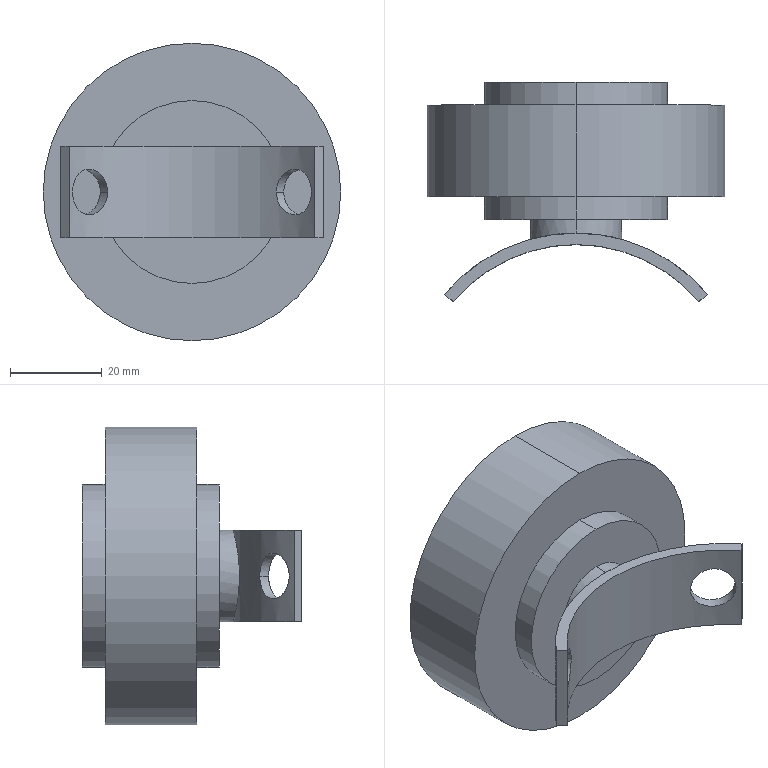Part | SolidWorks | features ICE 5, RevCut 2, Extrusion 1 | 1 solid | 26 faces | box 65 x 48.002 x 65 mm | volume 76467 mm3 | cylinder 17 | plane 9 | commonest cylinder face diameters 10 x4 20 x4 40 x4 65 x2 75 x2 70 x1
STEP:
#1=CARTESIAN_POINT('',(27.72,25.256,10.));
#2=VERTEX_POINT('',#1);
#3=CARTESIAN_POINT('',(20.059,31.684,10.));
#4=VERTEX_POINT('',#3);
#5=CARTESIAN_POINT('',(27.72,25.256,10.));
#6=CARTESIAN_POINT('',(27.72,25.256,9.669));
#7=CARTESIAN_POINT('',(27.697,25.281,9.344));
#8=CARTESIAN_POINT('',(27.632,25.351,8.864));
#9=CARTESIAN_POINT('',(27.605,25.381,8.706));
#10=CARTESIAN_POINT('',(27.54,25.452,8.392));
#11=CARTESIAN_POINT('',(27.502,25.493,8.235));
#12=CARTESIAN_POINT('',(27.373,25.632,7.781));
#13=CARTESIAN_POINT('',(27.267,25.745,7.494));
#14=CARTESIAN_POINT('',(27.015,26.009,6.951));
#15=CARTESIAN_POINT('',(26.868,26.162,6.694));
#16=CARTESIAN_POINT('',(26.543,26.491,6.233));
#17=CARTESIAN_POINT('',(26.364,26.67,6.027));
#18=CARTESIAN_POINT('',(25.971,27.052,5.661));
#19=CARTESIAN_POINT('',(25.761,27.253,5.506));
#20=CARTESIAN_POINT('',(25.32,27.663,5.257));
#21=CARTESIAN_POINT('',(25.086,27.876,5.16));
#22=CARTESIAN_POINT('',(24.602,28.304,5.032));
#23=CARTESIAN_POINT('',(24.356,28.516,5.));
#24=CARTESIAN_POINT('',(23.856,28.935,5.));
#25=CARTESIAN_POINT('',(23.599,29.145,5.032));
#26=CARTESIAN_POINT('',(23.097,29.545,5.16));
#27=CARTESIAN_POINT('',(22.85,29.736,5.255));
#28=CARTESIAN_POINT('',(22.487,30.01,5.443));
#29=CARTESIAN_POINT('',(22.367,30.1,5.514));
#30=CARTESIAN_POINT('',(22.133,30.272,5.669));
#31=CARTESIAN_POINT('',(22.02,30.354,5.753));
#32=CARTESIAN_POINT('',(21.689,30.592,6.024));
#33=CARTESIAN_POINT('',(21.482,30.738,6.231));
#34=CARTESIAN_POINT('',(21.096,31.004,6.697));
#35=CARTESIAN_POINT('',(20.924,31.12,6.95));
#36=CARTESIAN_POINT('',(20.697,31.272,7.355));
#37=CARTESIAN_POINT('',(20.626,31.318,7.495));
#38=CARTESIAN_POINT('',(20.495,31.404,7.785));
#39=CARTESIAN_POINT('',(20.436,31.443,7.935));
#40=CARTESIAN_POINT('',(20.276,31.546,8.389));
#41=CARTESIAN_POINT('',(20.196,31.597,8.7));
#42=CARTESIAN_POINT('',(20.087,31.666,9.342));
#43=CARTESIAN_POINT('',(20.059,31.684,9.673));
#44=CARTESIAN_POINT('',(20.059,31.684,10.));
#45=B_SPLINE_CURVE_WITH_KNOTS('',3,(#5,#6,#7,#8,#9,#10,#11,#12,#13,#14,#15,#16,#17,#18,#19,#20,#21,#22,#23,#24,#25,#26,#27,#28,#29,#30,#31,#32,#33,#34,#35,#36,#37,#38,#39,#40,#41,#42,#43,#44),.UNSPECIFIED.,.F.,.F.,(4,2,2,2,2,2,2,2,2,2,2,2,2,2,2,2,2,2,2,4),(0.,0.0009781,0.001467,0.001956,0.002934,0.003912,0.004891,0.005869,0.006847,0.007825,0.008803,0.009781,0.01027,0.01076,0.01174,0.01272,0.0132,0.01369,0.01467,0.01565),.UNSPECIFIED.);
#46=EDGE_CURVE('',#2,#4,#45,.T.);
#47=ORIENTED_EDGE('',*,*,#46,.T.);
#48=CARTESIAN_POINT('',(18.437,29.75,10.));
#49=VERTEX_POINT('',#48);
#50=CARTESIAN_POINT('',(13.962,24.418,10.));
#51=DIRECTION('',(-0.6428,-0.766,0.));
#52=VECTOR('',#51,1000.);
#53=LINE('',#50,#52);
#54=EDGE_CURVE('',#4,#49,#53,.T.);
#55=ORIENTED_EDGE('',*,*,#54,.T.);
#56=CARTESIAN_POINT('',(26.097,23.323,10.));
#57=VERTEX_POINT('',#56);
#58=CARTESIAN_POINT('',(18.437,29.75,10.));
#59=CARTESIAN_POINT('',(18.437,29.75,9.674));
#60=CARTESIAN_POINT('',(18.464,29.734,9.349));
#61=CARTESIAN_POINT('',(18.574,29.665,8.703));
#62=CARTESIAN_POINT('',(18.656,29.614,8.388));
#63=CARTESIAN_POINT('',(18.868,29.479,7.786));
#64=CARTESIAN_POINT('',(19.,29.394,7.495));
#65=CARTESIAN_POINT('',(19.308,29.193,6.949));
#66=CARTESIAN_POINT('',(19.481,29.078,6.697));
#67=CARTESIAN_POINT('',(19.864,28.818,6.236));
#68=CARTESIAN_POINT('',(20.076,28.671,6.025));
#69=CARTESIAN_POINT('',(20.519,28.356,5.662));
#70=CARTESIAN_POINT('',(20.751,28.186,5.509));
#71=CARTESIAN_POINT('',(21.115,27.914,5.32));
#72=CARTESIAN_POINT('',(21.24,27.819,5.264));
#73=CARTESIAN_POINT('',(21.489,27.627,5.168));
#74=CARTESIAN_POINT('',(21.613,27.53,5.129));
#75=CARTESIAN_POINT('',(21.989,27.232,5.033));
#76=CARTESIAN_POINT('',(22.242,27.026,5.));
#77=CARTESIAN_POINT('',(22.748,26.601,5.));
#78=CARTESIAN_POINT('',(22.994,26.389,5.032));
#79=CARTESIAN_POINT('',(23.473,25.964,5.159));
#80=CARTESIAN_POINT('',(23.708,25.749,5.255));
#81=CARTESIAN_POINT('',(24.15,25.335,5.506));
#82=CARTESIAN_POINT('',(24.358,25.135,5.659));
#83=CARTESIAN_POINT('',(24.746,24.753,6.021));
#84=CARTESIAN_POINT('',(24.928,24.57,6.232));
#85=CARTESIAN_POINT('',(25.251,24.238,6.692));
#86=CARTESIAN_POINT('',(25.394,24.087,6.943));
#87=CARTESIAN_POINT('',(25.647,23.818,7.49));
#88=CARTESIAN_POINT('',(25.753,23.703,7.78));
#89=CARTESIAN_POINT('',(25.923,23.517,8.381));
#90=CARTESIAN_POINT('',(25.988,23.444,8.696));
#91=CARTESIAN_POINT('',(26.075,23.347,9.342));
#92=CARTESIAN_POINT('',(26.097,23.323,9.669));
#93=CARTESIAN_POINT('',(26.097,23.323,10.));
#94=B_SPLINE_CURVE_WITH_KNOTS('',3,(#58,#59,#60,#61,#62,#63,#64,#65,#66,#67,#68,#69,#70,#71,#72,#73,#74,#75,#76,#77,#78,#79,#80,#81,#82,#83,#84,#85,#86,#87,#88,#89,#90,#91,#92,#93),.UNSPECIFIED.,.F.,.F.,(4,2,2,2,2,2,2,2,2,2,2,2,2,2,2,2,2,4),(0.01565,0.01663,0.01761,0.01859,0.01956,0.02054,0.02152,0.02201,0.0225,0.02348,0.02445,0.02543,0.02641,0.02739,0.02837,0.02934,0.03032,0.0313),.UNSPECIFIED.);
#95=EDGE_CURVE('',#49,#57,#94,.T.);
#96=ORIENTED_EDGE('',*,*,#95,.T.);
#97=CARTESIAN_POINT('',(21.623,17.991,10.));
#98=DIRECTION('',(-0.6428,-0.766,0.));
#99=VECTOR('',#98,1000.);
#100=LINE('',#97,#99);
#101=EDGE_CURVE('',#2,#57,#100,.T.);
#102=ORIENTED_EDGE('',*,*,#101,.F.);
#103=EDGE_LOOP('',(#47,#55,#96,#102));
#104=FACE_OUTER_BOUND('',#103,.T.);
#105=CARTESIAN_POINT('',(17.793,21.204,10.));
#106=DIRECTION('',(-0.6428,-0.766,0.));
#107=DIRECTION('',(0.766,-0.6428,0.));
#108=AXIS2_PLACEMENT_3D('',#105,#106,#107);
#109=CYLINDRICAL_SURFACE('',#108,5.);
#110=ADVANCED_FACE('',(#104),#109,.F.);
#111=CARTESIAN_POINT('',(-20.059,31.684,10.));
#112=VERTEX_POINT('',#111);
#113=CARTESIAN_POINT('',(-27.72,25.256,10.));
#114=VERTEX_POINT('',#113);
#115=CARTESIAN_POINT('',(-20.059,31.684,10.));
#116=CARTESIAN_POINT('',(-20.059,31.684,9.669));
#117=CARTESIAN_POINT('',(-20.087,31.667,9.344));
#118=CARTESIAN_POINT('',(-20.168,31.615,8.864));
#119=CARTESIAN_POINT('',(-20.202,31.593,8.706));
#120=CARTESIAN_POINT('',(-20.283,31.541,8.392));
#121=CARTESIAN_POINT('',(-20.33,31.511,8.235));
#122=CARTESIAN_POINT('',(-20.489,31.408,7.781));
#123=CARTESIAN_POINT('',(-20.619,31.323,7.494));
#124=CARTESIAN_POINT('',(-20.923,31.121,6.951));
#125=CARTESIAN_POINT('',(-21.099,31.002,6.694));
#126=CARTESIAN_POINT('',(-21.48,30.74,6.233));
#127=CARTESIAN_POINT('',(-21.687,30.594,6.027));
#128=CARTESIAN_POINT('',(-22.131,30.274,5.661));
#129=CARTESIAN_POINT('',(-22.366,30.102,5.506));
#130=CARTESIAN_POINT('',(-22.846,29.739,5.257));
#131=CARTESIAN_POINT('',(-23.096,29.545,5.16));
#132=CARTESIAN_POINT('',(-23.601,29.143,5.032));
#133=CARTESIAN_POINT('',(-23.853,28.938,5.));
#134=CARTESIAN_POINT('',(-24.353,28.518,5.));
#135=CARTESIAN_POINT('',(-24.605,28.301,5.032));
#136=CARTESIAN_POINT('',(-25.085,27.876,5.16));
#137=CARTESIAN_POINT('',(-25.316,27.666,5.255));
#138=CARTESIAN_POINT('',(-25.649,27.357,5.443));
#139=CARTESIAN_POINT('',(-25.759,27.254,5.514));
#140=CARTESIAN_POINT('',(-25.969,27.054,5.669));
#141=CARTESIAN_POINT('',(-26.07,26.956,5.753));
#142=CARTESIAN_POINT('',(-26.361,26.672,6.024));
#143=CARTESIAN_POINT('',(-26.541,26.493,6.231));
#144=CARTESIAN_POINT('',(-26.87,26.16,6.697));
#145=CARTESIAN_POINT('',(-27.014,26.01,6.95));
#146=CARTESIAN_POINT('',(-27.203,25.812,7.355));
#147=CARTESIAN_POINT('',(-27.261,25.751,7.495));
#148=CARTESIAN_POINT('',(-27.368,25.637,7.785));
#149=CARTESIAN_POINT('',(-27.416,25.585,7.935));
#150=CARTESIAN_POINT('',(-27.545,25.446,8.389));
#151=CARTESIAN_POINT('',(-27.61,25.376,8.7));
#152=CARTESIAN_POINT('',(-27.697,25.281,9.342));
#153=CARTESIAN_POINT('',(-27.72,25.256,9.673));
#154=CARTESIAN_POINT('',(-27.72,25.256,10.));
#155=B_SPLINE_CURVE_WITH_KNOTS('',3,(#115,#116,#117,#118,#119,#120,#121,#122,#123,#124,#125,#126,#127,#128,#129,#130,#131,#132,#133,#134,#135,#136,#137,#138,#139,#140,#141,#142,#143,#144,#145,#146,#147,#148,#149,#150,#151,#152,#153,#154),.UNSPECIFIED.,.F.,.F.,(4,2,2,2,2,2,2,2,2,2,2,2,2,2,2,2,2,2,2,4),(0.,0.0009781,0.001467,0.001956,0.002934,0.003912,0.004891,0.005869,0.006847,0.007825,0.008803,0.009781,0.01027,0.01076,0.01174,0.01272,0.0132,0.01369,0.01467,0.01565),.UNSPECIFIED.);
#156=EDGE_CURVE('',#112,#114,#155,.T.);
#157=ORIENTED_EDGE('',*,*,#156,.T.);
#158=CARTESIAN_POINT('',(-26.097,23.323,10.));
#159=VERTEX_POINT('',#158);
#160=CARTESIAN_POINT('',(-21.523,17.872,10.));
#161=DIRECTION('',(0.6428,-0.766,0.));
#162=VECTOR('',#161,1000.);
#163=LINE('',#160,#162);
#164=EDGE_CURVE('',#114,#159,#163,.T.);
#165=ORIENTED_EDGE('',*,*,#164,.T.);
#166=CARTESIAN_POINT('',(-18.437,29.75,10.));
#167=VERTEX_POINT('',#166);
#168=CARTESIAN_POINT('',(-26.097,23.323,10.));
#169=CARTESIAN_POINT('',(-26.097,23.323,9.674));
#170=CARTESIAN_POINT('',(-26.076,23.347,9.349));
#171=CARTESIAN_POINT('',(-25.989,23.443,8.703));
#172=CARTESIAN_POINT('',(-25.924,23.515,8.388));
#173=CARTESIAN_POINT('',(-25.755,23.7,7.786));
#174=CARTESIAN_POINT('',(-25.649,23.816,7.495));
#175=CARTESIAN_POINT('',(-25.397,24.084,6.949));
#176=CARTESIAN_POINT('',(-25.254,24.234,6.697));
#177=CARTESIAN_POINT('',(-24.931,24.566,6.236));
#178=CARTESIAN_POINT('',(-24.75,24.749,6.025));
#179=CARTESIAN_POINT('',(-24.362,25.131,5.662));
#180=CARTESIAN_POINT('',(-24.155,25.331,5.509));
#181=CARTESIAN_POINT('',(-23.823,25.642,5.32));
#182=CARTESIAN_POINT('',(-23.708,25.748,5.264));
#183=CARTESIAN_POINT('',(-23.476,25.959,5.168));
#184=CARTESIAN_POINT('',(-23.358,26.066,5.129));
#185=CARTESIAN_POINT('',(-23.,26.384,5.033));
#186=CARTESIAN_POINT('',(-22.753,26.597,5.));
#187=CARTESIAN_POINT('',(-22.247,27.022,5.));
#188=CARTESIAN_POINT('',(-21.995,27.227,5.032));
#189=CARTESIAN_POINT('',(-21.493,27.625,5.159));
#190=CARTESIAN_POINT('',(-21.241,27.819,5.255));
#191=CARTESIAN_POINT('',(-20.756,28.183,5.506));
#192=CARTESIAN_POINT('',(-20.524,28.352,5.659));
#193=CARTESIAN_POINT('',(-20.08,28.669,6.021));
#194=CARTESIAN_POINT('',(-19.868,28.815,6.232));
#195=CARTESIAN_POINT('',(-19.485,29.076,6.692));
#196=CARTESIAN_POINT('',(-19.311,29.191,6.943));
#197=CARTESIAN_POINT('',(-19.002,29.393,7.49));
#198=CARTESIAN_POINT('',(-18.871,29.477,7.78));
#199=CARTESIAN_POINT('',(-18.658,29.612,8.381));
#200=CARTESIAN_POINT('',(-18.575,29.664,8.696));
#201=CARTESIAN_POINT('',(-18.465,29.733,9.342));
#202=CARTESIAN_POINT('',(-18.437,29.75,9.669));
#203=CARTESIAN_POINT('',(-18.437,29.75,10.));
#204=B_SPLINE_CURVE_WITH_KNOTS('',3,(#168,#169,#170,#171,#172,#173,#174,#175,#176,#177,#178,#179,#180,#181,#182,#183,#184,#185,#186,#187,#188,#189,#190,#191,#192,#193,#194,#195,#196,#197,#198,#199,#200,#201,#202,#203),.UNSPECIFIED.,.F.,.F.,(4,2,2,2,2,2,2,2,2,2,2,2,2,2,2,2,2,4),(0.01565,0.01663,0.01761,0.01859,0.01956,0.02054,0.02152,0.02201,0.0225,0.02348,0.02445,0.02543,0.02641,0.02739,0.02837,0.02934,0.03032,0.0313),.UNSPECIFIED.);
#205=EDGE_CURVE('',#159,#167,#204,.T.);
#206=ORIENTED_EDGE('',*,*,#205,.T.);
#207=CARTESIAN_POINT('',(-13.863,24.3,10.));
#208=DIRECTION('',(0.6428,-0.766,0.));
#209=VECTOR('',#208,1000.);
#210=LINE('',#207,#209);
#211=EDGE_CURVE('',#112,#167,#210,.T.);
#212=ORIENTED_EDGE('',*,*,#211,.F.);
#213=EDGE_LOOP('',(#157,#165,#206,#212));
#214=FACE_OUTER_BOUND('',#213,.T.);
#215=CARTESIAN_POINT('',(-17.693,21.086,10.));
#216=DIRECTION('',(0.6428,-0.766,0.));
#217=DIRECTION('',(0.766,0.6428,0.));
#218=AXIS2_PLACEMENT_3D('',#215,#216,#217);
#219=CYLINDRICAL_SURFACE('',#218,5.);
#220=ADVANCED_FACE('',(#214),#219,.F.);
#221=CARTESIAN_POINT('',(0.,50.5,0.));
#222=VERTEX_POINT('',#221);
#223=CARTESIAN_POINT('',(0.,50.5,20.));
#224=VERTEX_POINT('',#223);
#225=CARTESIAN_POINT('',(0.,50.5,10.));
#226=DIRECTION('',(0.,1.,0.));
#227=DIRECTION('',(0.,0.,1.));
#228=AXIS2_PLACEMENT_3D('',#225,#226,#227);
#229=CIRCLE('',#228,10.);
#230=EDGE_CURVE('',#222,#224,#229,.T.);
#231=ORIENTED_EDGE('',*,*,#230,.F.);
#232=CARTESIAN_POINT('',(0.,70.5,0.));
#233=VERTEX_POINT('',#232);
#234=CARTESIAN_POINT('',(0.,50.5,0.));
#235=DIRECTION('',(0.,1.,0.));
#236=VECTOR('',#235,1000.);
#237=LINE('',#234,#236);
#238=EDGE_CURVE('',#222,#233,#237,.T.);
#239=ORIENTED_EDGE('',*,*,#238,.T.);
#240=CARTESIAN_POINT('',(0.,70.5,20.));
#241=VERTEX_POINT('',#240);
#242=CARTESIAN_POINT('',(0.,70.5,10.));
#243=DIRECTION('',(0.,1.,0.));
#244=DIRECTION('',(0.,0.,1.));
#245=AXIS2_PLACEMENT_3D('',#242,#243,#244);
#246=CIRCLE('',#245,10.);
#247=EDGE_CURVE('',#233,#241,#246,.T.);
#248=ORIENTED_EDGE('',*,*,#247,.T.);
#249=CARTESIAN_POINT('',(0.,50.5,20.));
#250=DIRECTION('',(0.,1.,0.));
#251=VECTOR('',#250,1000.);
#252=LINE('',#249,#251);
#253=EDGE_CURVE('',#224,#241,#252,.T.);
#254=ORIENTED_EDGE('',*,*,#253,.F.);
#255=EDGE_LOOP('',(#231,#239,#248,#254));
#256=FACE_OUTER_BOUND('',#255,.T.);
#257=CARTESIAN_POINT('',(0.,50.5,10.));
#258=DIRECTION('',(0.,1.,0.));
#259=DIRECTION('',(0.,0.,1.));
#260=AXIS2_PLACEMENT_3D('',#257,#258,#259);
#261=CYLINDRICAL_SURFACE('',#260,10.);
#262=ADVANCED_FACE('',(#256),#261,.F.);
#263=CARTESIAN_POINT('',(0.,70.5,30.));
#264=VERTEX_POINT('',#263);
#265=CARTESIAN_POINT('',(0.,70.5,-10.));
#266=VERTEX_POINT('',#265);
#267=CARTESIAN_POINT('',(0.,70.5,10.));
#268=DIRECTION('',(0.,1.,0.));
#269=DIRECTION('',(0.,0.,1.));
#270=AXIS2_PLACEMENT_3D('',#267,#268,#269);
#271=CIRCLE('',#270,20.);
#272=EDGE_CURVE('',#264,#266,#271,.T.);
#273=ORIENTED_EDGE('',*,*,#272,.F.);
#274=CARTESIAN_POINT('',(0.,65.5,30.));
#275=VERTEX_POINT('',#274);
#276=CARTESIAN_POINT('',(0.,70.5,30.));
#277=DIRECTION('',(0.,-1.,0.));
#278=VECTOR('',#277,1000.);
#279=LINE('',#276,#278);
#280=EDGE_CURVE('',#264,#275,#279,.T.);
#281=ORIENTED_EDGE('',*,*,#280,.T.);
#282=CARTESIAN_POINT('',(0.,65.5,-10.));
#283=VERTEX_POINT('',#282);
#284=CARTESIAN_POINT('',(0.,65.5,10.));
#285=DIRECTION('',(0.,1.,0.));
#286=DIRECTION('',(0.,0.,1.));
#287=AXIS2_PLACEMENT_3D('',#284,#285,#286);
#288=CIRCLE('',#287,20.);
#289=EDGE_CURVE('',#275,#283,#288,.T.);
#290=ORIENTED_EDGE('',*,*,#289,.T.);
#291=CARTESIAN_POINT('',(0.,70.5,-10.));
#292=DIRECTION('',(0.,-1.,0.));
#293=VECTOR('',#292,1000.);
#294=LINE('',#291,#293);
#295=EDGE_CURVE('',#266,#283,#294,.T.);
#296=ORIENTED_EDGE('',*,*,#295,.F.);
#297=EDGE_LOOP('',(#273,#281,#290,#296));
#298=FACE_OUTER_BOUND('',#297,.T.);
#299=CARTESIAN_POINT('',(0.,70.5,10.));
#300=DIRECTION('',(0.,-1.,0.));
#301=DIRECTION('',(0.,0.,-1.));
#302=AXIS2_PLACEMENT_3D('',#299,#300,#301);
#303=CYLINDRICAL_SURFACE('',#302,20.);
#304=ADVANCED_FACE('',(#298),#303,.T.);
#305=CARTESIAN_POINT('',(0.,65.5,42.5));
#306=VERTEX_POINT('',#305);
#307=CARTESIAN_POINT('',(0.,65.5,-22.5));
#308=VERTEX_POINT('',#307);
#309=CARTESIAN_POINT('',(0.,65.5,10.));
#310=DIRECTION('',(0.,1.,0.));
#311=DIRECTION('',(0.,0.,1.));
#312=AXIS2_PLACEMENT_3D('',#309,#310,#311);
#313=CIRCLE('',#312,32.5);
#314=EDGE_CURVE('',#306,#308,#313,.T.);
#315=ORIENTED_EDGE('',*,*,#314,.F.);
#316=CARTESIAN_POINT('',(0.,45.5,42.5));
#317=VERTEX_POINT('',#316);
#318=CARTESIAN_POINT('',(0.,65.5,42.5));
#319=DIRECTION('',(0.,-1.,0.));
#320=VECTOR('',#319,1000.);
#321=LINE('',#318,#320);
#322=EDGE_CURVE('',#306,#317,#321,.T.);
#323=ORIENTED_EDGE('',*,*,#322,.T.);
#324=CARTESIAN_POINT('',(0.,45.5,-22.5));
#325=VERTEX_POINT('',#324);
#326=CARTESIAN_POINT('',(0.,45.5,10.));
#327=DIRECTION('',(0.,1.,0.));
#328=DIRECTION('',(0.,0.,1.));
#329=AXIS2_PLACEMENT_3D('',#326,#327,#328);
#330=CIRCLE('',#329,32.5);
#331=EDGE_CURVE('',#317,#325,#330,.T.);
#332=ORIENTED_EDGE('',*,*,#331,.T.);
#333=CARTESIAN_POINT('',(0.,65.5,-22.5));
#334=DIRECTION('',(0.,-1.,0.));
#335=VECTOR('',#334,1000.);
#336=LINE('',#333,#335);
#337=EDGE_CURVE('',#308,#325,#336,.T.);
#338=ORIENTED_EDGE('',*,*,#337,.F.);
#339=EDGE_LOOP('',(#315,#323,#332,#338));
#340=FACE_OUTER_BOUND('',#339,.T.);
#341=CARTESIAN_POINT('',(0.,65.5,10.));
#342=DIRECTION('',(0.,-1.,0.));
#343=DIRECTION('',(0.,0.,-1.));
#344=AXIS2_PLACEMENT_3D('',#341,#342,#343);
#345=CYLINDRICAL_SURFACE('',#344,32.5);
#346=ADVANCED_FACE('',(#340),#345,.T.);
#347=CARTESIAN_POINT('',(0.,45.5,30.));
#348=VERTEX_POINT('',#347);
#349=CARTESIAN_POINT('',(0.,45.5,-10.));
#350=VERTEX_POINT('',#349);
#351=CARTESIAN_POINT('',(0.,45.5,10.));
#352=DIRECTION('',(0.,1.,0.));
#353=DIRECTION('',(0.,0.,1.));
#354=AXIS2_PLACEMENT_3D('',#351,#352,#353);
#355=CIRCLE('',#354,20.);
#356=EDGE_CURVE('',#348,#350,#355,.T.);
#357=ORIENTED_EDGE('',*,*,#356,.F.);
#358=CARTESIAN_POINT('',(0.,40.5,30.));
#359=VERTEX_POINT('',#358);
#360=CARTESIAN_POINT('',(0.,45.5,30.));
#361=DIRECTION('',(0.,-1.,0.));
#362=VECTOR('',#361,1000.);
#363=LINE('',#360,#362);
#364=EDGE_CURVE('',#348,#359,#363,.T.);
#365=ORIENTED_EDGE('',*,*,#364,.T.);
#366=CARTESIAN_POINT('',(0.,40.5,-10.));
#367=VERTEX_POINT('',#366);
#368=CARTESIAN_POINT('',(0.,40.5,10.));
#369=DIRECTION('',(0.,1.,0.));
#370=DIRECTION('',(0.,0.,1.));
#371=AXIS2_PLACEMENT_3D('',#368,#369,#370);
#372=CIRCLE('',#371,20.);
#373=EDGE_CURVE('',#359,#367,#372,.T.);
#374=ORIENTED_EDGE('',*,*,#373,.T.);
#375=CARTESIAN_POINT('',(0.,45.5,-10.));
#376=DIRECTION('',(0.,-1.,0.));
#377=VECTOR('',#376,1000.);
#378=LINE('',#375,#377);
#379=EDGE_CURVE('',#350,#367,#378,.T.);
#380=ORIENTED_EDGE('',*,*,#379,.F.);
#381=EDGE_LOOP('',(#357,#365,#374,#380));
#382=FACE_OUTER_BOUND('',#381,.T.);
#383=CARTESIAN_POINT('',(0.,45.5,10.));
#384=DIRECTION('',(0.,-1.,0.));
#385=DIRECTION('',(0.,0.,-1.));
#386=AXIS2_PLACEMENT_3D('',#383,#384,#385);
#387=CYLINDRICAL_SURFACE('',#386,20.);
#388=ADVANCED_FACE('',(#382),#387,.T.);
#389=CARTESIAN_POINT('',(0.,37.5,20.));
#390=VERTEX_POINT('',#389);
#391=CARTESIAN_POINT('',(0.,37.5,0.));
#392=VERTEX_POINT('',#391);
#393=CARTESIAN_POINT('',(0.,37.5,20.));
#394=CARTESIAN_POINT('',(0.664,37.5,20.));
#395=CARTESIAN_POINT('',(1.316,37.482,19.935));
#396=CARTESIAN_POINT('',(2.278,37.432,19.743));
#397=CARTESIAN_POINT('',(2.596,37.411,19.663));
#398=CARTESIAN_POINT('',(3.226,37.362,19.471));
#399=CARTESIAN_POINT('',(3.538,37.334,19.359));
#400=CARTESIAN_POINT('',(4.445,37.241,18.982));
#401=CARTESIAN_POINT('',(5.019,37.167,18.674));
#402=CARTESIAN_POINT('',(5.832,37.045,18.13));
#403=CARTESIAN_POINT('',(6.097,37.002,17.933));
#404=CARTESIAN_POINT('',(6.603,36.915,17.517));
#405=CARTESIAN_POINT('',(6.844,36.871,17.298));
#406=CARTESIAN_POINT('',(7.532,36.739,16.61));
#407=CARTESIAN_POINT('',(7.945,36.651,16.108));
#408=CARTESIAN_POINT('',(8.493,36.526,15.289));
#409=CARTESIAN_POINT('',(8.662,36.486,15.007));
#410=CARTESIAN_POINT('',(8.97,36.412,14.432));
#411=CARTESIAN_POINT('',(9.109,36.377,14.138));
#412=CARTESIAN_POINT('',(9.359,36.314,13.537));
#413=CARTESIAN_POINT('',(9.47,36.285,13.23));
#414=CARTESIAN_POINT('',(9.661,36.234,12.603));
#415=CARTESIAN_POINT('',(9.742,36.212,12.28));
#416=CARTESIAN_POINT('',(9.936,36.16,11.311));
#417=CARTESIAN_POINT('',(10.,36.142,10.66));
#418=CARTESIAN_POINT('',(10.,36.142,9.349));
#419=CARTESIAN_POINT('',(9.934,36.16,8.683));
#420=CARTESIAN_POINT('',(9.678,36.23,7.398));
#421=CARTESIAN_POINT('',(9.488,36.281,6.773));
#422=CARTESIAN_POINT('',(9.11,36.377,5.862));
#423=CARTESIAN_POINT('',(8.968,36.412,5.563));
#424=CARTESIAN_POINT('',(8.659,36.487,4.987));
#425=CARTESIAN_POINT('',(8.491,36.527,4.708));
#426=CARTESIAN_POINT('',(8.13,36.609,4.168));
#427=CARTESIAN_POINT('',(7.936,36.651,3.907));
#428=CARTESIAN_POINT('',(7.522,36.738,3.403));
#429=CARTESIAN_POINT('',(7.301,36.783,3.158));
#430=CARTESIAN_POINT('',(6.606,36.916,2.465));
#431=CARTESIAN_POINT('',(6.105,37.004,2.053));
#432=CARTESIAN_POINT('',(5.294,37.125,1.51));
#433=CARTESIAN_POINT('',(5.014,37.164,1.342));
#434=CARTESIAN_POINT('',(4.434,37.238,1.031));
#435=CARTESIAN_POINT('',(4.136,37.272,0.8896));
#436=CARTESIAN_POINT('',(3.231,37.365,0.5139));
#437=CARTESIAN_POINT('',(2.608,37.415,0.3236));
#438=CARTESIAN_POINT('',(1.641,37.465,0.13));
#439=CARTESIAN_POINT('',(1.311,37.479,0.08085));
#440=CARTESIAN_POINT('',(0.6549,37.496,0.01602));
#441=CARTESIAN_POINT('',(0.3272,37.5,0.));
#442=CARTESIAN_POINT('',(0.,37.5,0.));
#443=B_SPLINE_CURVE_WITH_KNOTS('',3,(#393,#394,#395,#396,#397,#398,#399,#400,#401,#402,#403,#404,#405,#406,#407,#408,#409,#410,#411,#412,#413,#414,#415,#416,#417,#418,#419,#420,#421,#422,#423,#424,#425,#426,#427,#428,#429,#430,#431,#432,#433,#434,#435,#436,#437,#438,#439,#440,#441,#442),.UNSPECIFIED.,.F.,.F.,(4,2,2,2,2,2,2,2,2,2,2,2,2,2,2,2,2,2,2,2,2,2,2,2,4),(0.,0.001963,0.002944,0.003926,0.005889,0.00687,0.007852,0.009815,0.0108,0.01178,0.01276,0.01374,0.0157,0.01767,0.01963,0.02061,0.02159,0.02257,0.02356,0.02552,0.0265,0.02748,0.02944,0.03043,0.03141),.UNSPECIFIED.);
#444=EDGE_CURVE('',#390,#392,#443,.T.);
#445=ORIENTED_EDGE('',*,*,#444,.T.);
#446=CARTESIAN_POINT('',(0.,40.5,0.));
#447=VERTEX_POINT('',#446);
#448=CARTESIAN_POINT('',(0.,22.496,0.));
#449=DIRECTION('',(0.,1.,0.));
#450=VECTOR('',#449,1000.);
#451=LINE('',#448,#450);
#452=EDGE_CURVE('',#392,#447,#451,.T.);
#453=ORIENTED_EDGE('',*,*,#452,.T.);
#454=CARTESIAN_POINT('',(0.,40.5,20.));
#455=VERTEX_POINT('',#454);
#456=CARTESIAN_POINT('',(0.,40.5,10.));
#457=DIRECTION('',(0.,1.,0.));
#458=DIRECTION('',(0.,0.,1.));
#459=AXIS2_PLACEMENT_3D('',#456,#457,#458);
#460=CIRCLE('',#459,10.);
#461=EDGE_CURVE('',#455,#447,#460,.T.);
#462=ORIENTED_EDGE('',*,*,#461,.F.);
#463=CARTESIAN_POINT('',(0.,22.496,20.));
#464=DIRECTION('',(0.,1.,0.));
#465=VECTOR('',#464,1000.);
#466=LINE('',#463,#465);
#467=EDGE_CURVE('',#390,#455,#466,.T.);
#468=ORIENTED_EDGE('',*,*,#467,.F.);
#469=EDGE_LOOP('',(#445,#453,#462,#468));
#470=FACE_OUTER_BOUND('',#469,.T.);
#471=CARTESIAN_POINT('',(0.,22.496,10.));
#472=DIRECTION('',(0.,1.,0.));
#473=DIRECTION('',(0.,0.,1.));
#474=AXIS2_PLACEMENT_3D('',#471,#472,#473);
#475=CYLINDRICAL_SURFACE('',#474,10.);
#476=ADVANCED_FACE('',(#470),#475,.T.);
#477=CARTESIAN_POINT('',(-26.812,22.498,0.));
#478=VERTEX_POINT('',#477);
#479=CARTESIAN_POINT('',(26.812,22.498,0.));
#480=VERTEX_POINT('',#479);
#481=CARTESIAN_POINT('',(0.,0.,0.));
#482=DIRECTION('',(0.,0.,-1.));
#483=DIRECTION('',(1.,0.,0.));
#484=AXIS2_PLACEMENT_3D('',#481,#482,#483);
#485=CIRCLE('',#484,35.);
#486=EDGE_CURVE('',#478,#480,#485,.T.);
#487=ORIENTED_EDGE('',*,*,#486,.T.);
#488=CARTESIAN_POINT('',(26.812,22.498,20.));
#489=VERTEX_POINT('',#488);
#490=CARTESIAN_POINT('',(26.812,22.498,20.));
#491=DIRECTION('',(0.,0.,-1.));
#492=VECTOR('',#491,1000.);
#493=LINE('',#490,#492);
#494=EDGE_CURVE('',#489,#480,#493,.T.);
#495=ORIENTED_EDGE('',*,*,#494,.F.);
#496=CARTESIAN_POINT('',(-26.812,22.498,20.));
#497=VERTEX_POINT('',#496);
#498=CARTESIAN_POINT('',(0.,0.,20.));
#499=DIRECTION('',(0.,0.,-1.));
#500=DIRECTION('',(1.,0.,0.));
#501=AXIS2_PLACEMENT_3D('',#498,#499,#500);
#502=CIRCLE('',#501,35.);
#503=EDGE_CURVE('',#497,#489,#502,.T.);
#504=ORIENTED_EDGE('',*,*,#503,.F.);
#505=CARTESIAN_POINT('',(-26.812,22.498,20.));
#506=DIRECTION('',(0.,0.,-1.));
#507=VECTOR('',#506,1000.);
#508=LINE('',#505,#507);
#509=EDGE_CURVE('',#497,#478,#508,.T.);
#510=ORIENTED_EDGE('',*,*,#509,.T.);
#511=EDGE_LOOP('',(#487,#495,#504,#510));
#512=FACE_OUTER_BOUND('',#511,.T.);
#513=CARTESIAN_POINT('',(-18.437,29.75,10.));
#514=CARTESIAN_POINT('',(-18.437,29.75,10.331));
#515=CARTESIAN_POINT('',(-18.465,29.733,10.656));
#516=CARTESIAN_POINT('',(-18.546,29.682,11.136));
#517=CARTESIAN_POINT('',(-18.58,29.661,11.294));
#518=CARTESIAN_POINT('',(-18.662,29.61,11.609));
#519=CARTESIAN_POINT('',(-18.71,29.58,11.765));
#520=CARTESIAN_POINT('',(-18.87,29.478,12.219));
#521=CARTESIAN_POINT('',(-19.,29.394,12.506));
#522=CARTESIAN_POINT('',(-19.306,29.194,13.049));
#523=CARTESIAN_POINT('',(-19.483,29.077,13.306));
#524=CARTESIAN_POINT('',(-19.866,28.816,13.767));
#525=CARTESIAN_POINT('',(-20.074,28.673,13.973));
#526=CARTESIAN_POINT('',(-20.52,28.355,14.339));
#527=CARTESIAN_POINT('',(-20.756,28.183,14.494));
#528=CARTESIAN_POINT('',(-21.238,27.822,14.743));
#529=CARTESIAN_POINT('',(-21.488,27.629,14.84));
#530=CARTESIAN_POINT('',(-21.994,27.228,14.968));
#531=CARTESIAN_POINT('',(-22.246,27.023,15.));
#532=CARTESIAN_POINT('',(-22.746,26.603,15.));
#533=CARTESIAN_POINT('',(-22.997,26.386,14.967));
#534=CARTESIAN_POINT('',(-23.477,25.96,14.84));
#535=CARTESIAN_POINT('',(-23.708,25.749,14.745));
#536=CARTESIAN_POINT('',(-24.04,25.438,14.557));
#537=CARTESIAN_POINT('',(-24.149,25.335,14.486));
#538=CARTESIAN_POINT('',(-24.358,25.134,14.331));
#539=CARTESIAN_POINT('',(-24.458,25.036,14.247));
#540=CARTESIAN_POINT('',(-24.749,24.75,13.976));
#541=CARTESIAN_POINT('',(-24.927,24.57,13.769));
#542=CARTESIAN_POINT('',(-25.254,24.234,13.303));
#543=CARTESIAN_POINT('',(-25.397,24.083,13.051));
#544=CARTESIAN_POINT('',(-25.647,23.818,12.509));
#545=CARTESIAN_POINT('',(-25.754,23.701,12.217));
#546=CARTESIAN_POINT('',(-25.925,23.515,11.612));
#547=CARTESIAN_POINT('',(-25.989,23.444,11.3));
#548=CARTESIAN_POINT('',(-26.075,23.347,10.658));
#549=CARTESIAN_POINT('',(-26.097,23.323,10.327));
#550=CARTESIAN_POINT('',(-26.097,23.323,10.));
#551=B_SPLINE_CURVE_WITH_KNOTS('',3,(#513,#514,#515,#516,#517,#518,#519,#520,#521,#522,#523,#524,#525,#526,#527,#528,#529,#530,#531,#532,#533,#534,#535,#536,#537,#538,#539,#540,#541,#542,#543,#544,#545,#546,#547,#548,#549,#550),.UNSPECIFIED.,.F.,.F.,(4,2,2,2,2,2,2,2,2,2,2,2,2,2,2,2,2,2,4),(0.,0.0009783,0.001467,0.001957,0.002935,0.003913,0.004891,0.00587,0.006848,0.007826,0.008804,0.009783,0.01027,0.01076,0.01174,0.01272,0.0137,0.01467,0.01565),.UNSPECIFIED.);
#552=EDGE_CURVE('',#167,#159,#551,.T.);
#553=ORIENTED_EDGE('',*,*,#552,.F.);
#554=ORIENTED_EDGE('',*,*,#205,.F.);
#555=EDGE_LOOP('',(#553,#554));
#556=FACE_BOUND('',#555,.T.);
#557=CARTESIAN_POINT('',(26.097,23.323,10.));
#558=CARTESIAN_POINT('',(26.097,23.323,10.331));
#559=CARTESIAN_POINT('',(26.075,23.347,10.656));
#560=CARTESIAN_POINT('',(26.011,23.419,11.136));
#561=CARTESIAN_POINT('',(25.984,23.449,11.294));
#562=CARTESIAN_POINT('',(25.919,23.52,11.609));
#563=CARTESIAN_POINT('',(25.881,23.562,11.765));
#564=CARTESIAN_POINT('',(25.753,23.702,12.219));
#565=CARTESIAN_POINT('',(25.648,23.816,12.506));
#566=CARTESIAN_POINT('',(25.398,24.083,13.049));
#567=CARTESIAN_POINT('',(25.252,24.236,13.306));
#568=CARTESIAN_POINT('',(24.929,24.568,13.767));
#569=CARTESIAN_POINT('',(24.751,24.748,13.973));
#570=CARTESIAN_POINT('',(24.361,25.132,14.339));
#571=CARTESIAN_POINT('',(24.151,25.334,14.494));
#572=CARTESIAN_POINT('',(23.711,25.746,14.743));
#573=CARTESIAN_POINT('',(23.478,25.959,14.84));
#574=CARTESIAN_POINT('',(22.995,26.388,14.968));
#575=CARTESIAN_POINT('',(22.749,26.6,15.));
#576=CARTESIAN_POINT('',(22.249,27.02,15.));
#577=CARTESIAN_POINT('',(21.992,27.23,14.967));
#578=CARTESIAN_POINT('',(21.489,27.629,14.84));
#579=CARTESIAN_POINT('',(21.241,27.819,14.745));
#580=CARTESIAN_POINT('',(20.877,28.092,14.557));
#581=CARTESIAN_POINT('',(20.756,28.181,14.486));
#582=CARTESIAN_POINT('',(20.522,28.352,14.331));
#583=CARTESIAN_POINT('',(20.408,28.434,14.247));
#584=CARTESIAN_POINT('',(20.077,28.671,13.976));
#585=CARTESIAN_POINT('',(19.868,28.815,13.769));
#586=CARTESIAN_POINT('',(19.481,29.079,13.303));
#587=CARTESIAN_POINT('',(19.307,29.193,13.051));
#588=CARTESIAN_POINT('',(19.002,29.393,12.509));
#589=CARTESIAN_POINT('',(18.869,29.478,12.217));
#590=CARTESIAN_POINT('',(18.656,29.614,11.612));
#591=CARTESIAN_POINT('',(18.575,29.665,11.3));
#592=CARTESIAN_POINT('',(18.465,29.733,10.658));
#593=CARTESIAN_POINT('',(18.437,29.75,10.327));
#594=CARTESIAN_POINT('',(18.437,29.75,10.));
#595=B_SPLINE_CURVE_WITH_KNOTS('',3,(#557,#558,#559,#560,#561,#562,#563,#564,#565,#566,#567,#568,#569,#570,#571,#572,#573,#574,#575,#576,#577,#578,#579,#580,#581,#582,#583,#584,#585,#586,#587,#588,#589,#590,#591,#592,#593,#594),.UNSPECIFIED.,.F.,.F.,(4,2,2,2,2,2,2,2,2,2,2,2,2,2,2,2,2,2,4),(0.,0.0009783,0.001467,0.001957,0.002935,0.003913,0.004891,0.00587,0.006848,0.007826,0.008804,0.009783,0.01027,0.01076,0.01174,0.01272,0.0137,0.01467,0.01565),.UNSPECIFIED.);
#596=EDGE_CURVE('',#57,#49,#595,.T.);
#597=ORIENTED_EDGE('',*,*,#596,.F.);
#598=ORIENTED_EDGE('',*,*,#95,.F.);
#599=EDGE_LOOP('',(#597,#598));
#600=FACE_BOUND('',#599,.T.);
#601=CARTESIAN_POINT('',(0.,0.,20.));
#602=DIRECTION('',(0.,0.,-1.));
#603=DIRECTION('',(-1.,0.,0.));
#604=AXIS2_PLACEMENT_3D('',#601,#602,#603);
#605=CYLINDRICAL_SURFACE('',#604,35.);
#606=ADVANCED_FACE('',(#512,#556,#600),#605,.F.);
#607=CARTESIAN_POINT('',(28.727,24.105,0.));
#608=VERTEX_POINT('',#607);
#609=CARTESIAN_POINT('',(0.,0.,0.));
#610=DIRECTION('',(0.,0.,1.));
#611=DIRECTION('',(1.,0.,0.));
#612=AXIS2_PLACEMENT_3D('',#609,#610,#611);
#613=CIRCLE('',#612,37.5);
#614=EDGE_CURVE('',#608,#392,#613,.T.);
#615=ORIENTED_EDGE('',*,*,#614,.T.);
#616=ORIENTED_EDGE('',*,*,#444,.F.);
#617=CARTESIAN_POINT('',(28.727,24.105,20.));
#618=VERTEX_POINT('',#617);
#619=CARTESIAN_POINT('',(0.,0.,20.));
#620=DIRECTION('',(0.,0.,1.));
#621=DIRECTION('',(1.,0.,0.));
#622=AXIS2_PLACEMENT_3D('',#619,#620,#621);
#623=CIRCLE('',#622,37.5);
#624=EDGE_CURVE('',#618,#390,#623,.T.);
#625=ORIENTED_EDGE('',*,*,#624,.F.);
#626=CARTESIAN_POINT('',(28.727,24.105,20.));
#627=DIRECTION('',(0.,0.,-1.));
#628=VECTOR('',#627,1000.);
#629=LINE('',#626,#628);
#630=EDGE_CURVE('',#618,#608,#629,.T.);
#631=ORIENTED_EDGE('',*,*,#630,.T.);
#632=EDGE_LOOP('',(#615,#616,#625,#631));
#633=FACE_OUTER_BOUND('',#632,.T.);
#634=ORIENTED_EDGE('',*,*,#46,.F.);
#635=CARTESIAN_POINT('',(20.059,31.684,10.));
#636=CARTESIAN_POINT('',(20.059,31.684,10.326));
#637=CARTESIAN_POINT('',(20.086,31.667,10.651));
#638=CARTESIAN_POINT('',(20.195,31.598,11.297));
#639=CARTESIAN_POINT('',(20.277,31.545,11.612));
#640=CARTESIAN_POINT('',(20.488,31.409,12.214));
#641=CARTESIAN_POINT('',(20.619,31.323,12.505));
#642=CARTESIAN_POINT('',(20.924,31.12,13.051));
#643=CARTESIAN_POINT('',(21.096,31.004,13.303));
#644=CARTESIAN_POINT('',(21.477,30.741,13.764));
#645=CARTESIAN_POINT('',(21.688,30.593,13.975));
#646=CARTESIAN_POINT('',(22.13,30.275,14.338));
#647=CARTESIAN_POINT('',(22.361,30.105,14.491));
#648=CARTESIAN_POINT('',(22.724,29.831,14.68));
#649=CARTESIAN_POINT('',(22.848,29.736,14.736));
#650=CARTESIAN_POINT('',(23.097,29.544,14.832));
#651=CARTESIAN_POINT('',(23.221,29.446,14.871));
#652=CARTESIAN_POINT('',(23.597,29.147,14.967));
#653=CARTESIAN_POINT('',(23.849,28.941,15.));
#654=CARTESIAN_POINT('',(24.355,28.516,15.));
#655=CARTESIAN_POINT('',(24.601,28.304,14.968));
#656=CARTESIAN_POINT('',(25.081,27.88,14.841));
#657=CARTESIAN_POINT('',(25.316,27.666,14.745));
#658=CARTESIAN_POINT('',(25.76,27.254,14.495));
#659=CARTESIAN_POINT('',(25.968,27.055,14.341));
#660=CARTESIAN_POINT('',(26.359,26.675,13.979));
#661=CARTESIAN_POINT('',(26.541,26.493,13.768));
#662=CARTESIAN_POINT('',(26.866,26.163,13.308));
#663=CARTESIAN_POINT('',(27.011,26.013,13.057));
#664=CARTESIAN_POINT('',(27.265,25.747,12.51));
#665=CARTESIAN_POINT('',(27.372,25.633,12.22));
#666=CARTESIAN_POINT('',(27.544,25.448,11.619));
#667=CARTESIAN_POINT('',(27.609,25.377,11.304));
#668=CARTESIAN_POINT('',(27.697,25.28,10.658));
#669=CARTESIAN_POINT('',(27.72,25.256,10.331));
#670=CARTESIAN_POINT('',(27.72,25.256,10.));
#671=B_SPLINE_CURVE_WITH_KNOTS('',3,(#635,#636,#637,#638,#639,#640,#641,#642,#643,#644,#645,#646,#647,#648,#649,#650,#651,#652,#653,#654,#655,#656,#657,#658,#659,#660,#661,#662,#663,#664,#665,#666,#667,#668,#669,#670),.UNSPECIFIED.,.F.,.F.,(4,2,2,2,2,2,2,2,2,2,2,2,2,2,2,2,2,4),(0.01565,0.01663,0.01761,0.01858,0.01956,0.02054,0.02152,0.02201,0.02249,0.02347,0.02445,0.02543,0.02641,0.02738,0.02836,0.02934,0.03032,0.0313),.UNSPECIFIED.);
#672=EDGE_CURVE('',#4,#2,#671,.T.);
#673=ORIENTED_EDGE('',*,*,#672,.F.);
#674=EDGE_LOOP('',(#634,#673));
#675=FACE_BOUND('',#674,.T.);
#676=CARTESIAN_POINT('',(0.,0.,20.));
#677=DIRECTION('',(0.,0.,-1.));
#678=DIRECTION('',(-1.,0.,0.));
#679=AXIS2_PLACEMENT_3D('',#676,#677,#678);
#680=CYLINDRICAL_SURFACE('',#679,37.5);
#681=ADVANCED_FACE('',(#633,#675),#680,.T.);
#682=CARTESIAN_POINT('',(-28.727,24.105,20.));
#683=VERTEX_POINT('',#682);
#684=CARTESIAN_POINT('',(0.,0.,20.));
#685=DIRECTION('',(0.,0.,1.));
#686=DIRECTION('',(1.,0.,0.));
#687=AXIS2_PLACEMENT_3D('',#684,#685,#686);
#688=CIRCLE('',#687,37.5);
#689=EDGE_CURVE('',#390,#683,#688,.T.);
#690=ORIENTED_EDGE('',*,*,#689,.F.);
#691=CARTESIAN_POINT('',(0.,37.5,0.));
#692=CARTESIAN_POINT('',(-0.6543,37.5,0.));
#693=CARTESIAN_POINT('',(-1.308,37.483,0.06379));
#694=CARTESIAN_POINT('',(-2.607,37.415,0.3231));
#695=CARTESIAN_POINT('',(-3.232,37.365,0.5143));
#696=CARTESIAN_POINT('',(-4.136,37.272,0.8895));
#697=CARTESIAN_POINT('',(-4.431,37.238,1.029));
#698=CARTESIAN_POINT('',(-5.01,37.165,1.339));
#699=CARTESIAN_POINT('',(-5.293,37.126,1.509));
#700=CARTESIAN_POINT('',(-6.106,37.004,2.054));
#701=CARTESIAN_POINT('',(-6.608,36.916,2.466));
#702=CARTESIAN_POINT('',(-7.299,36.783,3.157));
#703=CARTESIAN_POINT('',(-7.521,36.739,3.401));
#704=CARTESIAN_POINT('',(-7.936,36.651,3.907));
#705=CARTESIAN_POINT('',(-8.13,36.609,4.168));
#706=CARTESIAN_POINT('',(-8.672,36.485,4.978));
#707=CARTESIAN_POINT('',(-8.98,36.41,5.551));
#708=CARTESIAN_POINT('',(-9.486,36.281,6.768));
#709=CARTESIAN_POINT('',(-9.677,36.23,7.396));
#710=CARTESIAN_POINT('',(-9.869,36.178,8.357));
#711=CARTESIAN_POINT('',(-9.918,36.165,8.68));
#712=CARTESIAN_POINT('',(-9.983,36.147,9.335));
#713=CARTESIAN_POINT('',(-10.,36.142,9.668));
#714=CARTESIAN_POINT('',(-10.,36.142,10.657));
#715=CARTESIAN_POINT('',(-9.936,36.16,11.308));
#716=CARTESIAN_POINT('',(-9.744,36.212,12.272));
#717=CARTESIAN_POINT('',(-9.664,36.234,12.592));
#718=CARTESIAN_POINT('',(-9.472,36.284,13.225));
#719=CARTESIAN_POINT('',(-9.361,36.313,13.533));
#720=CARTESIAN_POINT('',(-8.985,36.409,14.437));
#721=CARTESIAN_POINT('',(-8.678,36.484,15.012));
#722=CARTESIAN_POINT('',(-8.131,36.608,15.83));
#723=CARTESIAN_POINT('',(-7.935,36.651,16.094));
#724=CARTESIAN_POINT('',(-7.522,36.738,16.597));
#725=CARTESIAN_POINT('',(-7.304,36.783,16.838));
#726=CARTESIAN_POINT('',(-6.846,36.871,17.297));
#727=CARTESIAN_POINT('',(-6.605,36.915,17.515));
#728=CARTESIAN_POINT('',(-6.101,37.001,17.93));
#729=CARTESIAN_POINT('',(-5.836,37.044,18.127));
#730=CARTESIAN_POINT('',(-5.02,37.166,18.673));
#731=CARTESIAN_POINT('',(-4.447,37.24,18.98));
#732=CARTESIAN_POINT('',(-3.243,37.364,19.482));
#733=CARTESIAN_POINT('',(-2.606,37.415,19.677));
#734=CARTESIAN_POINT('',(-1.318,37.482,19.935));
#735=CARTESIAN_POINT('',(-0.6638,37.5,20.));
#736=CARTESIAN_POINT('',(0.,37.5,20.));
#737=B_SPLINE_CURVE_WITH_KNOTS('',3,(#691,#692,#693,#694,#695,#696,#697,#698,#699,#700,#701,#702,#703,#704,#705,#706,#707,#708,#709,#710,#711,#712,#713,#714,#715,#716,#717,#718,#719,#720,#721,#722,#723,#724,#725,#726,#727,#728,#729,#730,#731,#732,#733,#734,#735,#736),.UNSPECIFIED.,.F.,.F.,(4,2,2,2,2,2,2,2,2,2,2,2,2,2,2,2,2,2,2,2,2,2,4),(0.03141,0.03337,0.03533,0.03631,0.03729,0.03926,0.04024,0.04122,0.04318,0.04514,0.04613,0.04711,0.04907,0.05005,0.05103,0.05299,0.05398,0.05496,0.05594,0.05692,0.05888,0.06084,0.06281),.UNSPECIFIED.);
#738=EDGE_CURVE('',#392,#390,#737,.T.);
#739=ORIENTED_EDGE('',*,*,#738,.F.);
#740=CARTESIAN_POINT('',(-28.727,24.105,0.));
#741=VERTEX_POINT('',#740);
#742=CARTESIAN_POINT('',(0.,0.,0.));
#743=DIRECTION('',(0.,0.,1.));
#744=DIRECTION('',(1.,0.,0.));
#745=AXIS2_PLACEMENT_3D('',#742,#743,#744);
#746=CIRCLE('',#745,37.5);
#747=EDGE_CURVE('',#392,#741,#746,.T.);
#748=ORIENTED_EDGE('',*,*,#747,.T.);
#749=CARTESIAN_POINT('',(-28.727,24.105,20.));
#750=DIRECTION('',(0.,0.,-1.));
#751=VECTOR('',#750,1000.);
#752=LINE('',#749,#751);
#753=EDGE_CURVE('',#683,#741,#752,.T.);
#754=ORIENTED_EDGE('',*,*,#753,.F.);
#755=EDGE_LOOP('',(#690,#739,#748,#754));
#756=FACE_OUTER_BOUND('',#755,.T.);
#757=ORIENTED_EDGE('',*,*,#156,.F.);
#758=CARTESIAN_POINT('',(-27.72,25.256,10.));
#759=CARTESIAN_POINT('',(-27.72,25.256,10.326));
#760=CARTESIAN_POINT('',(-27.698,25.28,10.651));
#761=CARTESIAN_POINT('',(-27.611,25.375,11.297));
#762=CARTESIAN_POINT('',(-27.545,25.447,11.612));
#763=CARTESIAN_POINT('',(-27.374,25.63,12.214));
#764=CARTESIAN_POINT('',(-27.267,25.745,12.505));
#765=CARTESIAN_POINT('',(-27.014,26.01,13.051));
#766=CARTESIAN_POINT('',(-26.87,26.16,13.303));
#767=CARTESIAN_POINT('',(-26.545,26.489,13.764));
#768=CARTESIAN_POINT('',(-26.362,26.671,13.975));
#769=CARTESIAN_POINT('',(-25.973,27.051,14.338));
#770=CARTESIAN_POINT('',(-25.765,27.249,14.491));
#771=CARTESIAN_POINT('',(-25.432,27.559,14.68));
#772=CARTESIAN_POINT('',(-25.317,27.665,14.736));
#773=CARTESIAN_POINT('',(-25.084,27.876,14.832));
#774=CARTESIAN_POINT('',(-24.966,27.982,14.871));
#775=CARTESIAN_POINT('',(-24.607,28.299,14.967));
#776=CARTESIAN_POINT('',(-24.36,28.512,15.));
#777=CARTESIAN_POINT('',(-23.854,28.937,15.));
#778=CARTESIAN_POINT('',(-23.602,29.143,14.968));
#779=CARTESIAN_POINT('',(-23.102,29.541,14.841));
#780=CARTESIAN_POINT('',(-22.85,29.736,14.745));
#781=CARTESIAN_POINT('',(-22.366,30.101,14.495));
#782=CARTESIAN_POINT('',(-22.135,30.272,14.341));
#783=CARTESIAN_POINT('',(-21.692,30.59,13.979));
#784=CARTESIAN_POINT('',(-21.481,30.739,13.768));
#785=CARTESIAN_POINT('',(-21.1,31.001,13.308));
#786=CARTESIAN_POINT('',(-20.928,31.118,13.057));
#787=CARTESIAN_POINT('',(-20.621,31.322,12.51));
#788=CARTESIAN_POINT('',(-20.49,31.407,12.22));
#789=CARTESIAN_POINT('',(-20.279,31.544,11.619));
#790=CARTESIAN_POINT('',(-20.197,31.597,11.304));
#791=CARTESIAN_POINT('',(-20.087,31.667,10.658));
#792=CARTESIAN_POINT('',(-20.059,31.684,10.331));
#793=CARTESIAN_POINT('',(-20.059,31.684,10.));
#794=B_SPLINE_CURVE_WITH_KNOTS('',3,(#758,#759,#760,#761,#762,#763,#764,#765,#766,#767,#768,#769,#770,#771,#772,#773,#774,#775,#776,#777,#778,#779,#780,#781,#782,#783,#784,#785,#786,#787,#788,#789,#790,#791,#792,#793),.UNSPECIFIED.,.F.,.F.,(4,2,2,2,2,2,2,2,2,2,2,2,2,2,2,2,2,4),(0.01565,0.01663,0.01761,0.01858,0.01956,0.02054,0.02152,0.02201,0.02249,0.02347,0.02445,0.02543,0.02641,0.02738,0.02836,0.02934,0.03032,0.0313),.UNSPECIFIED.);
#795=EDGE_CURVE('',#114,#112,#794,.T.);
#796=ORIENTED_EDGE('',*,*,#795,.F.);
#797=EDGE_LOOP('',(#757,#796));
#798=FACE_BOUND('',#797,.T.);
#799=CARTESIAN_POINT('',(0.,0.,20.));
#800=DIRECTION('',(0.,0.,-1.));
#801=DIRECTION('',(-1.,0.,0.));
#802=AXIS2_PLACEMENT_3D('',#799,#800,#801);
#803=CYLINDRICAL_SURFACE('',#802,37.5);
#804=ADVANCED_FACE('',(#756,#798),#803,.T.);
#805=CARTESIAN_POINT('',(26.812,22.498,0.));
#806=DIRECTION('',(0.766,0.6428,0.));
#807=VECTOR('',#806,1000.);
#808=LINE('',#805,#807);
#809=EDGE_CURVE('',#480,#608,#808,.T.);
#810=ORIENTED_EDGE('',*,*,#809,.T.);
#811=ORIENTED_EDGE('',*,*,#630,.F.);
#812=CARTESIAN_POINT('',(26.812,22.498,20.));
#813=DIRECTION('',(0.766,0.6428,0.));
#814=VECTOR('',#813,1000.);
#815=LINE('',#812,#814);
#816=EDGE_CURVE('',#489,#618,#815,.T.);
#817=ORIENTED_EDGE('',*,*,#816,.F.);
#818=ORIENTED_EDGE('',*,*,#494,.T.);
#819=EDGE_LOOP('',(#810,#811,#817,#818));
#820=FACE_OUTER_BOUND('',#819,.T.);
#821=CARTESIAN_POINT('',(26.812,22.498,20.));
#822=DIRECTION('',(-0.6428,0.766,0.));
#823=DIRECTION('',(-0.766,-0.6428,0.));
#824=AXIS2_PLACEMENT_3D('',#821,#822,#823);
#825=PLANE('',#824);
#826=ADVANCED_FACE('',(#820),#825,.F.);
#827=CARTESIAN_POINT('',(-26.812,22.498,0.));
#828=DIRECTION('',(0.766,-0.6428,0.));
#829=VECTOR('',#828,1000.);
#830=LINE('',#827,#829);
#831=EDGE_CURVE('',#741,#478,#830,.T.);
#832=ORIENTED_EDGE('',*,*,#831,.T.);
#833=ORIENTED_EDGE('',*,*,#509,.F.);
#834=CARTESIAN_POINT('',(-26.812,22.498,20.));
#835=DIRECTION('',(0.766,-0.6428,0.));
#836=VECTOR('',#835,1000.);
#837=LINE('',#834,#836);
#838=EDGE_CURVE('',#683,#497,#837,.T.);
#839=ORIENTED_EDGE('',*,*,#838,.F.);
#840=ORIENTED_EDGE('',*,*,#753,.T.);
#841=EDGE_LOOP('',(#832,#833,#839,#840));
#842=FACE_OUTER_BOUND('',#841,.T.);
#843=CARTESIAN_POINT('',(-26.812,22.498,20.));
#844=DIRECTION('',(0.6428,0.766,0.));
#845=DIRECTION('',(-0.766,0.6428,0.));
#846=AXIS2_PLACEMENT_3D('',#843,#844,#845);
#847=PLANE('',#846);
#848=ADVANCED_FACE('',(#842),#847,.F.);
#849=ORIENTED_EDGE('',*,*,#503,.T.);
#850=ORIENTED_EDGE('',*,*,#816,.T.);
#851=ORIENTED_EDGE('',*,*,#624,.T.);
#852=ORIENTED_EDGE('',*,*,#689,.T.);
#853=ORIENTED_EDGE('',*,*,#838,.T.);
#854=EDGE_LOOP('',(#849,#850,#851,#852,#853));
#855=FACE_OUTER_BOUND('',#854,.T.);
#856=CARTESIAN_POINT('',(0.,0.,20.));
#857=DIRECTION('',(0.,0.,1.));
#858=DIRECTION('',(1.,0.,0.));
#859=AXIS2_PLACEMENT_3D('',#856,#857,#858);
#860=PLANE('',#859);
#861=ADVANCED_FACE('',(#855),#860,.T.);
#862=ORIENTED_EDGE('',*,*,#486,.F.);
#863=ORIENTED_EDGE('',*,*,#831,.F.);
#864=ORIENTED_EDGE('',*,*,#747,.F.);
#865=ORIENTED_EDGE('',*,*,#614,.F.);
#866=ORIENTED_EDGE('',*,*,#809,.F.);
#867=EDGE_LOOP('',(#862,#863,#864,#865,#866));
#868=FACE_OUTER_BOUND('',#867,.T.);
#869=CARTESIAN_POINT('',(0.,0.,0.));
#870=DIRECTION('',(0.,0.,1.));
#871=DIRECTION('',(1.,0.,0.));
#872=AXIS2_PLACEMENT_3D('',#869,#870,#871);
#873=PLANE('',#872);
#874=ADVANCED_FACE('',(#868),#873,.F.);
#875=ORIENTED_EDGE('',*,*,#452,.F.);
#876=ORIENTED_EDGE('',*,*,#738,.T.);
#877=ORIENTED_EDGE('',*,*,#467,.T.);
#878=CARTESIAN_POINT('',(0.,40.5,10.));
#879=DIRECTION('',(0.,1.,0.));
#880=DIRECTION('',(0.,0.,1.));
#881=AXIS2_PLACEMENT_3D('',#878,#879,#880);
#882=CIRCLE('',#881,10.);
#883=EDGE_CURVE('',#447,#455,#882,.T.);
#884=ORIENTED_EDGE('',*,*,#883,.F.);
#885=EDGE_LOOP('',(#875,#876,#877,#884));
#886=FACE_OUTER_BOUND('',#885,.T.);
#887=CARTESIAN_POINT('',(0.,22.496,10.));
#888=DIRECTION('',(0.,1.,0.));
#889=DIRECTION('',(0.,0.,1.));
#890=AXIS2_PLACEMENT_3D('',#887,#888,#889);
#891=CYLINDRICAL_SURFACE('',#890,10.);
#892=ADVANCED_FACE('',(#886),#891,.T.);
#893=ORIENTED_EDGE('',*,*,#364,.F.);
#894=CARTESIAN_POINT('',(0.,45.5,10.));
#895=DIRECTION('',(0.,1.,0.));
#896=DIRECTION('',(0.,0.,1.));
#897=AXIS2_PLACEMENT_3D('',#894,#895,#896);
#898=CIRCLE('',#897,20.);
#899=EDGE_CURVE('',#350,#348,#898,.T.);
#900=ORIENTED_EDGE('',*,*,#899,.F.);
#901=ORIENTED_EDGE('',*,*,#379,.T.);
#902=CARTESIAN_POINT('',(0.,40.5,10.));
#903=DIRECTION('',(0.,1.,0.));
#904=DIRECTION('',(0.,0.,1.));
#905=AXIS2_PLACEMENT_3D('',#902,#903,#904);
#906=CIRCLE('',#905,20.);
#907=EDGE_CURVE('',#367,#359,#906,.T.);
#908=ORIENTED_EDGE('',*,*,#907,.T.);
#909=EDGE_LOOP('',(#893,#900,#901,#908));
#910=FACE_OUTER_BOUND('',#909,.T.);
#911=CARTESIAN_POINT('',(0.,45.5,10.));
#912=DIRECTION('',(0.,-1.,0.));
#913=DIRECTION('',(0.,0.,-1.));
#914=AXIS2_PLACEMENT_3D('',#911,#912,#913);
#915=CYLINDRICAL_SURFACE('',#914,20.);
#916=ADVANCED_FACE('',(#910),#915,.T.);
#917=ORIENTED_EDGE('',*,*,#461,.T.);
#918=ORIENTED_EDGE('',*,*,#883,.T.);
#919=EDGE_LOOP('',(#917,#918));
#920=FACE_BOUND('',#919,.T.);
#921=ORIENTED_EDGE('',*,*,#907,.F.);
#922=ORIENTED_EDGE('',*,*,#373,.F.);
#923=EDGE_LOOP('',(#921,#922));
#924=FACE_OUTER_BOUND('',#923,.T.);
#925=CARTESIAN_POINT('',(0.,40.5,10.));
#926=DIRECTION('',(0.,1.,0.));
#927=DIRECTION('',(0.,0.,1.));
#928=AXIS2_PLACEMENT_3D('',#925,#926,#927);
#929=PLANE('',#928);
#930=ADVANCED_FACE('',(#920,#924),#929,.F.);
#931=ORIENTED_EDGE('',*,*,#322,.F.);
#932=CARTESIAN_POINT('',(0.,65.5,10.));
#933=DIRECTION('',(0.,1.,0.));
#934=DIRECTION('',(0.,0.,1.));
#935=AXIS2_PLACEMENT_3D('',#932,#933,#934);
#936=CIRCLE('',#935,32.5);
#937=EDGE_CURVE('',#308,#306,#936,.T.);
#938=ORIENTED_EDGE('',*,*,#937,.F.);
#939=ORIENTED_EDGE('',*,*,#337,.T.);
#940=CARTESIAN_POINT('',(0.,45.5,10.));
#941=DIRECTION('',(0.,1.,0.));
#942=DIRECTION('',(0.,0.,1.));
#943=AXIS2_PLACEMENT_3D('',#940,#941,#942);
#944=CIRCLE('',#943,32.5);
#945=EDGE_CURVE('',#325,#317,#944,.T.);
#946=ORIENTED_EDGE('',*,*,#945,.T.);
#947=EDGE_LOOP('',(#931,#938,#939,#946));
#948=FACE_OUTER_BOUND('',#947,.T.);
#949=CARTESIAN_POINT('',(0.,65.5,10.));
#950=DIRECTION('',(0.,-1.,0.));
#951=DIRECTION('',(0.,0.,-1.));
#952=AXIS2_PLACEMENT_3D('',#949,#950,#951);
#953=CYLINDRICAL_SURFACE('',#952,32.5);
#954=ADVANCED_FACE('',(#948),#953,.T.);
#955=CARTESIAN_POINT('',(0.,65.5,10.));
#956=DIRECTION('',(0.,1.,0.));
#957=DIRECTION('',(0.,0.,1.));
#958=AXIS2_PLACEMENT_3D('',#955,#956,#957);
#959=CIRCLE('',#958,20.);
#960=EDGE_CURVE('',#283,#275,#959,.T.);
#961=ORIENTED_EDGE('',*,*,#960,.F.);
#962=ORIENTED_EDGE('',*,*,#289,.F.);
#963=EDGE_LOOP('',(#961,#962));
#964=FACE_BOUND('',#963,.T.);
#965=ORIENTED_EDGE('',*,*,#937,.T.);
#966=ORIENTED_EDGE('',*,*,#314,.T.);
#967=EDGE_LOOP('',(#965,#966));
#968=FACE_OUTER_BOUND('',#967,.T.);
#969=CARTESIAN_POINT('',(0.,65.5,10.));
#970=DIRECTION('',(0.,1.,0.));
#971=DIRECTION('',(0.,0.,1.));
#972=AXIS2_PLACEMENT_3D('',#969,#970,#971);
#973=PLANE('',#972);
#974=ADVANCED_FACE('',(#964,#968),#973,.T.);
#975=ORIENTED_EDGE('',*,*,#899,.T.);
#976=ORIENTED_EDGE('',*,*,#356,.T.);
#977=EDGE_LOOP('',(#975,#976));
#978=FACE_BOUND('',#977,.T.);
#979=ORIENTED_EDGE('',*,*,#945,.F.);
#980=ORIENTED_EDGE('',*,*,#331,.F.);
#981=EDGE_LOOP('',(#979,#980));
#982=FACE_OUTER_BOUND('',#981,.T.);
#983=CARTESIAN_POINT('',(0.,45.5,10.));
#984=DIRECTION('',(0.,1.,0.));
#985=DIRECTION('',(0.,0.,1.));
#986=AXIS2_PLACEMENT_3D('',#983,#984,#985);
#987=PLANE('',#986);
#988=ADVANCED_FACE('',(#978,#982),#987,.F.);
#989=ORIENTED_EDGE('',*,*,#280,.F.);
#990=CARTESIAN_POINT('',(0.,70.5,10.));
#991=DIRECTION('',(0.,1.,0.));
#992=DIRECTION('',(0.,0.,1.));
#993=AXIS2_PLACEMENT_3D('',#990,#991,#992);
#994=CIRCLE('',#993,20.);
#995=EDGE_CURVE('',#266,#264,#994,.T.);
#996=ORIENTED_EDGE('',*,*,#995,.F.);
#997=ORIENTED_EDGE('',*,*,#295,.T.);
#998=ORIENTED_EDGE('',*,*,#960,.T.);
#999=EDGE_LOOP('',(#989,#996,#997,#998));
#1000=FACE_OUTER_BOUND('',#999,.T.);
#1001=CARTESIAN_POINT('',(0.,70.5,10.));
#1002=DIRECTION('',(0.,-1.,0.));
#1003=DIRECTION('',(0.,0.,-1.));
#1004=AXIS2_PLACEMENT_3D('',#1001,#1002,#1003);
#1005=CYLINDRICAL_SURFACE('',#1004,20.);
#1006=ADVANCED_FACE('',(#1000),#1005,.T.);
#1007=CARTESIAN_POINT('',(0.,70.5,10.));
#1008=DIRECTION('',(0.,1.,0.));
#1009=DIRECTION('',(0.,0.,1.));
#1010=AXIS2_PLACEMENT_3D('',#1007,#1008,#1009);
#1011=CIRCLE('',#1010,10.);
#1012=EDGE_CURVE('',#241,#233,#1011,.T.);
#1013=ORIENTED_EDGE('',*,*,#1012,.F.);
#1014=ORIENTED_EDGE('',*,*,#247,.F.);
#1015=EDGE_LOOP('',(#1013,#1014));
#1016=FACE_BOUND('',#1015,.T.);
#1017=ORIENTED_EDGE('',*,*,#995,.T.);
#1018=ORIENTED_EDGE('',*,*,#272,.T.);
#1019=EDGE_LOOP('',(#1017,#1018));
#1020=FACE_OUTER_BOUND('',#1019,.T.);
#1021=CARTESIAN_POINT('',(0.,70.5,10.));
#1022=DIRECTION('',(0.,1.,0.));
#1023=DIRECTION('',(0.,0.,1.));
#1024=AXIS2_PLACEMENT_3D('',#1021,#1022,#1023);
#1025=PLANE('',#1024);
#1026=ADVANCED_FACE('',(#1016,#1020),#1025,.T.);
#1027=ORIENTED_EDGE('',*,*,#238,.F.);
#1028=CARTESIAN_POINT('',(0.,50.5,10.));
#1029=DIRECTION('',(0.,1.,0.));
#1030=DIRECTION('',(0.,0.,1.));
#1031=AXIS2_PLACEMENT_3D('',#1028,#1029,#1030);
#1032=CIRCLE('',#1031,10.);
#1033=EDGE_CURVE('',#224,#222,#1032,.T.);
#1034=ORIENTED_EDGE('',*,*,#1033,.F.);
#1035=ORIENTED_EDGE('',*,*,#253,.T.);
#1036=ORIENTED_EDGE('',*,*,#1012,.T.);
#1037=EDGE_LOOP('',(#1027,#1034,#1035,#1036));
#1038=FACE_OUTER_BOUND('',#1037,.T.);
#1039=CARTESIAN_POINT('',(0.,50.5,10.));
#1040=DIRECTION('',(0.,1.,0.));
#1041=DIRECTION('',(0.,0.,1.));
#1042=AXIS2_PLACEMENT_3D('',#1039,#1040,#1041);
#1043=CYLINDRICAL_SURFACE('',#1042,10.);
#1044=ADVANCED_FACE('',(#1038),#1043,.F.);
#1045=ORIENTED_EDGE('',*,*,#1033,.T.);
#1046=ORIENTED_EDGE('',*,*,#230,.T.);
#1047=EDGE_LOOP('',(#1045,#1046));
#1048=FACE_OUTER_BOUND('',#1047,.T.);
#1049=CARTESIAN_POINT('',(0.,50.5,10.));
#1050=DIRECTION('',(0.,1.,0.));
#1051=DIRECTION('',(0.,0.,1.));
#1052=AXIS2_PLACEMENT_3D('',#1049,#1050,#1051);
#1053=PLANE('',#1052);
#1054=ADVANCED_FACE('',(#1048),#1053,.T.);
#1055=ORIENTED_EDGE('',*,*,#164,.F.);
#1056=ORIENTED_EDGE('',*,*,#795,.T.);
#1057=ORIENTED_EDGE('',*,*,#211,.T.);
#1058=ORIENTED_EDGE('',*,*,#552,.T.);
#1059=EDGE_LOOP('',(#1055,#1056,#1057,#1058));
#1060=FACE_OUTER_BOUND('',#1059,.T.);
#1061=CARTESIAN_POINT('',(-17.693,21.086,10.));
#1062=DIRECTION('',(0.6428,-0.766,0.));
#1063=DIRECTION('',(0.766,0.6428,0.));
#1064=AXIS2_PLACEMENT_3D('',#1061,#1062,#1063);
#1065=CYLINDRICAL_SURFACE('',#1064,5.);
#1066=ADVANCED_FACE('',(#1060),#1065,.F.);
#1067=ORIENTED_EDGE('',*,*,#54,.F.);
#1068=ORIENTED_EDGE('',*,*,#672,.T.);
#1069=ORIENTED_EDGE('',*,*,#101,.T.);
#1070=ORIENTED_EDGE('',*,*,#596,.T.);
#1071=EDGE_LOOP('',(#1067,#1068,#1069,#1070));
#1072=FACE_OUTER_BOUND('',#1071,.T.);
#1073=CARTESIAN_POINT('',(17.793,21.204,10.));
#1074=DIRECTION('',(-0.6428,-0.766,0.));
#1075=DIRECTION('',(0.766,-0.6428,0.));
#1076=AXIS2_PLACEMENT_3D('',#1073,#1074,#1075);
#1077=CYLINDRICAL_SURFACE('',#1076,5.);
#1078=ADVANCED_FACE('',(#1072),#1077,.F.);
#1079=CLOSED_SHELL('',(#110,#220,#262,#304,#346,#388,#476,#606,#681,#804,#826,#848,#861,#874,#892,#916,#930,#954,#974,#988,#1006,#1026,#1044,#1054,#1066,#1078));
#1080=MANIFOLD_SOLID_BREP('',#1079);
#1081=CARTESIAN_POINT('',(0.,0.,0.));
#1082=DIRECTION('',(0.,0.,1.));
#1083=DIRECTION('',(1.,0.,0.));
#1084=AXIS2_PLACEMENT_3D('',#1081,#1082,#1083);
#1085=(LENGTH_UNIT()NAMED_UNIT(*)SI_UNIT(.MILLI.,.METRE.));
#1086=UNCERTAINTY_MEASURE_WITH_UNIT(LENGTH_MEASURE(0.00001),#1085,'','');
#1087=(NAMED_UNIT(*)PLANE_ANGLE_UNIT()SI_UNIT($,.RADIAN.));
#1088=(NAMED_UNIT(*)SI_UNIT($,.STERADIAN.)SOLID_ANGLE_UNIT());
#1089=(GEOMETRIC_REPRESENTATION_CONTEXT(3)GLOBAL_UNCERTAINTY_ASSIGNED_CONTEXT((#1086))GLOBAL_UNIT_ASSIGNED_CONTEXT((#1085,#1087,#1088))REPRESENTATION_CONTEXT('',''));
#1090=ADVANCED_BREP_SHAPE_REPRESENTATION('',(#1080,#1084),#1089);